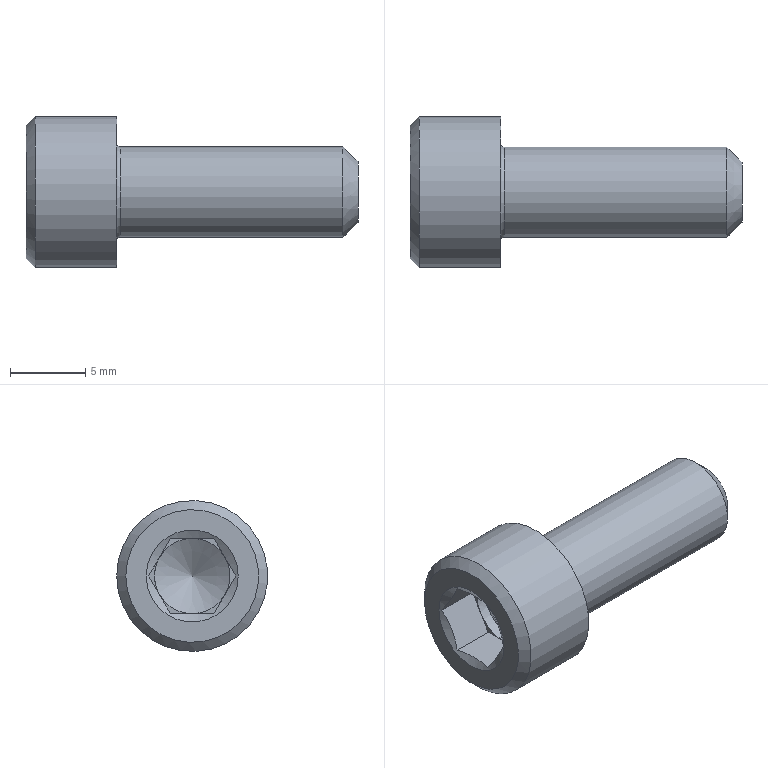Part | STEP file | Винт М6-6gx16 ГОСТ 11738-84 | 1 solid | 23 faces | box 22 x 10 x 10 mm | volume 820.968 mm3 | plane 15 | cone 4 | cylinder 3 | torus 1 | commonest cylinder face diameters 5 x1 6 x1 10 x1
STEP:
#1=CARTESIAN_POINT('',(-6.,4.4,0.));
#2=VERTEX_POINT('',#1);
#3=CARTESIAN_POINT('',(-6.,0.,0.));
#4=DIRECTION('',(1.,0.,0.));
#5=DIRECTION('',(0.,1.,0.));
#6=AXIS2_PLACEMENT_3D('',#3,#4,#5);
#7=CIRCLE('',#6,4.4);
#8=EDGE_CURVE('',#2,#2,#7,.T.);
#9=ORIENTED_EDGE('',*,*,#8,.F.);
#10=EDGE_LOOP('',(#9));
#11=FACE_BOUND('',#10,.T.);
#12=CARTESIAN_POINT('',(-6.,3.05,0.));
#13=VERTEX_POINT('',#12);
#14=CARTESIAN_POINT('',(-6.,0.,0.));
#15=DIRECTION('',(1.,0.,0.));
#16=DIRECTION('',(0.,1.,0.));
#17=AXIS2_PLACEMENT_3D('',#14,#15,#16);
#18=CIRCLE('',#17,3.05);
#19=EDGE_CURVE('',#13,#13,#18,.T.);
#20=ORIENTED_EDGE('',*,*,#19,.T.);
#21=EDGE_LOOP('',(#20));
#22=FACE_BOUND('',#21,.T.);
#23=CARTESIAN_POINT('',(-6.,0.,0.));
#24=DIRECTION('',(-1.,0.,0.));
#25=DIRECTION('',(0.,1.,0.));
#26=AXIS2_PLACEMENT_3D('',#23,#24,#25);
#27=PLANE('',#26);
#28=ADVANCED_FACE('',(#11,#22),#27,.T.);
#29=CARTESIAN_POINT('',(-5.906,1.443,-2.5));
#30=VERTEX_POINT('',#29);
#31=CARTESIAN_POINT('',(-5.906,-1.443,-2.5));
#32=VERTEX_POINT('',#31);
#33=CARTESIAN_POINT('',(-5.906,1.443,-2.5));
#34=CARTESIAN_POINT('',(-5.9,1.424,-2.5));
#35=CARTESIAN_POINT('',(-5.89,1.389,-2.5));
#36=CARTESIAN_POINT('',(-5.88,1.351,-2.5));
#37=CARTESIAN_POINT('',(-5.867,1.304,-2.5));
#38=CARTESIAN_POINT('',(-5.848,1.232,-2.5));
#39=CARTESIAN_POINT('',(-5.827,1.146,-2.5));
#40=CARTESIAN_POINT('',(-5.803,1.043,-2.5));
#41=CARTESIAN_POINT('',(-5.774,0.909,-2.5));
#42=CARTESIAN_POINT('',(-5.75,0.7773,-2.5));
#43=CARTESIAN_POINT('',(-5.728,0.6356,-2.5));
#44=CARTESIAN_POINT('',(-5.711,0.5115,-2.5));
#45=CARTESIAN_POINT('',(-5.699,0.3892,-2.5));
#46=CARTESIAN_POINT('',(-5.692,0.2947,-2.5));
#47=CARTESIAN_POINT('',(-5.688,0.2222,-2.5));
#48=CARTESIAN_POINT('',(-5.684,0.1323,-2.5));
#49=CARTESIAN_POINT('',(-5.683,0.05578,-2.5));
#50=CARTESIAN_POINT('',(-5.682,-0.001577,-2.5));
#51=CARTESIAN_POINT('',(-5.683,-0.03169,-2.5));
#52=CARTESIAN_POINT('',(-5.683,-0.0738,-2.5));
#53=CARTESIAN_POINT('',(-5.684,-0.1276,-2.5));
#54=CARTESIAN_POINT('',(-5.687,-0.2055,-2.5));
#55=CARTESIAN_POINT('',(-5.692,-0.2839,-2.5));
#56=CARTESIAN_POINT('',(-5.696,-0.3444,-2.5));
#57=CARTESIAN_POINT('',(-5.7,-0.3959,-2.5));
#58=CARTESIAN_POINT('',(-5.705,-0.4472,-2.5));
#59=CARTESIAN_POINT('',(-5.713,-0.5148,-2.5));
#60=CARTESIAN_POINT('',(-5.722,-0.5907,-2.5));
#61=CARTESIAN_POINT('',(-5.73,-0.6507,-2.5));
#62=CARTESIAN_POINT('',(-5.738,-0.7005,-2.5));
#63=CARTESIAN_POINT('',(-5.746,-0.7498,-2.5));
#64=CARTESIAN_POINT('',(-5.757,-0.8136,-2.5));
#65=CARTESIAN_POINT('',(-5.77,-0.8864,-2.5));
#66=CARTESIAN_POINT('',(-5.785,-0.9583,-2.5));
#67=CARTESIAN_POINT('',(-5.8,-1.03,-2.5));
#68=CARTESIAN_POINT('',(-5.812,-1.084,-2.5));
#69=CARTESIAN_POINT('',(-5.823,-1.131,-2.5));
#70=CARTESIAN_POINT('',(-5.834,-1.177,-2.5));
#71=CARTESIAN_POINT('',(-5.85,-1.239,-2.5));
#72=CARTESIAN_POINT('',(-5.868,-1.307,-2.5));
#73=CARTESIAN_POINT('',(-5.882,-1.361,-2.5));
#74=CARTESIAN_POINT('',(-5.895,-1.406,-2.5));
#75=CARTESIAN_POINT('',(-5.902,-1.429,-2.5));
#76=CARTESIAN_POINT('',(-5.906,-1.443,-2.5));
#77=B_SPLINE_CURVE_WITH_KNOTS('',3,(#33,#34,#35,#36,#37,#38,#39,#40,#41,#42,#43,#44,#45,#46,#47,#48,#49,#50,#51,#52,#53,#54,#55,#56,#57,#58,#59,#60,#61,#62,#63,#64,#65,#66,#67,#68,#69,#70,#71,#72,#73,#74,#75,#76),.UNSPECIFIED.,.F.,.F.,(4,1,1,1,1,1,1,1,1,1,1,1,1,1,1,1,1,1,1,1,1,1,1,1,1,1,1,1,1,1,1,1,1,1,1,1,1,1,1,1,1,4),(0.,0.02097,0.03685,0.04095,0.07015,0.1134,0.1316,0.1778,0.2541,0.2686,0.3246,0.3823,0.3943,0.4217,0.4566,0.4863,0.5,0.5153,0.5171,0.5431,0.5703,0.5969,0.6234,0.6325,0.6498,0.6761,0.7022,0.7281,0.7381,0.7538,0.7792,0.8044,0.8294,0.8543,0.8789,0.8866,0.9033,0.9276,0.9518,0.9759,0.9843,1.),.UNSPECIFIED.);
#78=EDGE_CURVE('',#30,#32,#77,.T.);
#79=ORIENTED_EDGE('',*,*,#78,.T.);
#80=CARTESIAN_POINT('',(-3.,-1.443,-2.5));
#81=VERTEX_POINT('',#80);
#82=CARTESIAN_POINT('',(-3.,-1.443,-2.5));
#83=DIRECTION('',(-1.,0.,0.));
#84=VECTOR('',#83,1.);
#85=LINE('',#82,#84);
#86=EDGE_CURVE('',#81,#32,#85,.T.);
#87=ORIENTED_EDGE('',*,*,#86,.F.);
#88=CARTESIAN_POINT('',(-3.,0.,-2.5));
#89=VERTEX_POINT('',#88);
#90=CARTESIAN_POINT('',(-3.,0.,-2.5));
#91=DIRECTION('',(0.,-1.,0.));
#92=VECTOR('',#91,1.);
#93=LINE('',#90,#92);
#94=EDGE_CURVE('',#89,#81,#93,.T.);
#95=ORIENTED_EDGE('',*,*,#94,.F.);
#96=CARTESIAN_POINT('',(-3.,1.443,-2.5));
#97=VERTEX_POINT('',#96);
#98=CARTESIAN_POINT('',(-3.,1.443,-2.5));
#99=DIRECTION('',(0.,-1.,0.));
#100=VECTOR('',#99,1.);
#101=LINE('',#98,#100);
#102=EDGE_CURVE('',#97,#89,#101,.T.);
#103=ORIENTED_EDGE('',*,*,#102,.F.);
#104=CARTESIAN_POINT('',(-3.,1.443,-2.5));
#105=DIRECTION('',(-1.,0.,0.));
#106=VECTOR('',#105,1.);
#107=LINE('',#104,#106);
#108=EDGE_CURVE('',#97,#30,#107,.T.);
#109=ORIENTED_EDGE('',*,*,#108,.T.);
#110=EDGE_LOOP('',(#79,#87,#95,#103,#109));
#111=FACE_BOUND('',#110,.T.);
#112=CARTESIAN_POINT('',(-3.,1.443,-2.5));
#113=DIRECTION('',(0.,0.,-1.));
#114=DIRECTION('',(0.,-1.,0.));
#115=AXIS2_PLACEMENT_3D('',#112,#113,#114);
#116=PLANE('',#115);
#117=ADVANCED_FACE('',(#111),#116,.F.);
#118=CARTESIAN_POINT('',(-5.906,-2.887,0.));
#119=VERTEX_POINT('',#118);
#120=CARTESIAN_POINT('',(-5.906,-1.443,-2.5));
#121=CARTESIAN_POINT('',(-5.9,-1.453,-2.483));
#122=CARTESIAN_POINT('',(-5.889,-1.472,-2.45));
#123=CARTESIAN_POINT('',(-5.871,-1.505,-2.392));
#124=CARTESIAN_POINT('',(-5.848,-1.549,-2.317));
#125=CARTESIAN_POINT('',(-5.816,-1.614,-2.204));
#126=CARTESIAN_POINT('',(-5.777,-1.702,-2.052));
#127=CARTESIAN_POINT('',(-5.74,-1.803,-1.877));
#128=CARTESIAN_POINT('',(-5.713,-1.902,-1.705));
#129=CARTESIAN_POINT('',(-5.697,-1.984,-1.564));
#130=CARTESIAN_POINT('',(-5.688,-2.048,-1.453));
#131=CARTESIAN_POINT('',(-5.684,-2.099,-1.365));
#132=CARTESIAN_POINT('',(-5.683,-2.137,-1.298));
#133=CARTESIAN_POINT('',(-5.682,-2.166,-1.249));
#134=CARTESIAN_POINT('',(-5.683,-2.194,-1.201));
#135=CARTESIAN_POINT('',(-5.684,-2.228,-1.141));
#136=CARTESIAN_POINT('',(-5.687,-2.268,-1.072));
#137=CARTESIAN_POINT('',(-5.692,-2.307,-1.004));
#138=CARTESIAN_POINT('',(-5.697,-2.346,-0.9371));
#139=CARTESIAN_POINT('',(-5.704,-2.384,-0.8704));
#140=CARTESIAN_POINT('',(-5.713,-2.422,-0.8041));
#141=CARTESIAN_POINT('',(-5.722,-2.46,-0.7384));
#142=CARTESIAN_POINT('',(-5.733,-2.498,-0.6734));
#143=CARTESIAN_POINT('',(-5.744,-2.535,-0.609));
#144=CARTESIAN_POINT('',(-5.757,-2.572,-0.5454));
#145=CARTESIAN_POINT('',(-5.77,-2.608,-0.4824));
#146=CARTESIAN_POINT('',(-5.785,-2.644,-0.4201));
#147=CARTESIAN_POINT('',(-5.8,-2.68,-0.3584));
#148=CARTESIAN_POINT('',(-5.816,-2.715,-0.2974));
#149=CARTESIAN_POINT('',(-5.832,-2.75,-0.237));
#150=CARTESIAN_POINT('',(-5.85,-2.784,-0.1771));
#151=CARTESIAN_POINT('',(-5.868,-2.819,-0.1177));
#152=CARTESIAN_POINT('',(-5.886,-2.853,-0.05869));
#153=CARTESIAN_POINT('',(-5.899,-2.875,-0.01952));
#154=CARTESIAN_POINT('',(-5.906,-2.887,0.));
#155=B_SPLINE_CURVE_WITH_KNOTS('',3,(#120,#121,#122,#123,#124,#125,#126,#127,#128,#129,#130,#131,#132,#133,#134,#135,#136,#137,#138,#139,#140,#141,#142,#143,#144,#145,#146,#147,#148,#149,#150,#151,#152,#153,#154),.UNSPECIFIED.,.F.,.F.,(4,1,1,1,1,1,1,1,1,1,1,1,1,1,1,1,1,1,1,1,1,1,1,1,1,1,1,1,1,1,1,1,4),(0.,0.02097,0.04095,0.07015,0.1134,0.1778,0.2541,0.3246,0.3823,0.4217,0.4566,0.4863,0.5,0.5153,0.5431,0.5703,0.5969,0.6234,0.6498,0.6761,0.7022,0.7281,0.7538,0.7792,0.8044,0.8294,0.8543,0.8789,0.9033,0.9276,0.9518,0.9759,1.),.UNSPECIFIED.);
#156=EDGE_CURVE('',#32,#119,#155,.T.);
#157=ORIENTED_EDGE('',*,*,#156,.T.);
#158=CARTESIAN_POINT('',(-3.,-2.887,0.));
#159=VERTEX_POINT('',#158);
#160=CARTESIAN_POINT('',(-3.,-2.887,0.));
#161=DIRECTION('',(-1.,0.,0.));
#162=VECTOR('',#161,1.);
#163=LINE('',#160,#162);
#164=EDGE_CURVE('',#159,#119,#163,.T.);
#165=ORIENTED_EDGE('',*,*,#164,.F.);
#166=CARTESIAN_POINT('',(-3.,-2.165,-1.25));
#167=VERTEX_POINT('',#166);
#168=CARTESIAN_POINT('',(-3.,-2.165,-1.25));
#169=DIRECTION('',(0.,-0.5,0.866));
#170=VECTOR('',#169,1.);
#171=LINE('',#168,#170);
#172=EDGE_CURVE('',#167,#159,#171,.T.);
#173=ORIENTED_EDGE('',*,*,#172,.F.);
#174=CARTESIAN_POINT('',(-3.,-1.443,-2.5));
#175=DIRECTION('',(0.,-0.5,0.866));
#176=VECTOR('',#175,1.);
#177=LINE('',#174,#176);
#178=EDGE_CURVE('',#81,#167,#177,.T.);
#179=ORIENTED_EDGE('',*,*,#178,.F.);
#180=ORIENTED_EDGE('',*,*,#86,.T.);
#181=EDGE_LOOP('',(#157,#165,#173,#179,#180));
#182=FACE_BOUND('',#181,.T.);
#183=CARTESIAN_POINT('',(-3.,-1.443,-2.5));
#184=DIRECTION('',(0.,-0.866,-0.5));
#185=DIRECTION('',(0.,-0.5,0.866));
#186=AXIS2_PLACEMENT_3D('',#183,#184,#185);
#187=PLANE('',#186);
#188=ADVANCED_FACE('',(#182),#187,.F.);
#189=CARTESIAN_POINT('',(-5.906,-1.443,2.5));
#190=VERTEX_POINT('',#189);
#191=CARTESIAN_POINT('',(-5.906,-2.887,0.));
#192=CARTESIAN_POINT('',(-5.9,-2.877,0.01704));
#193=CARTESIAN_POINT('',(-5.889,-2.858,0.05036));
#194=CARTESIAN_POINT('',(-5.871,-2.825,0.1076));
#195=CARTESIAN_POINT('',(-5.848,-2.781,0.1832));
#196=CARTESIAN_POINT('',(-5.816,-2.716,0.2956));
#197=CARTESIAN_POINT('',(-5.777,-2.628,0.4476));
#198=CARTESIAN_POINT('',(-5.74,-2.527,0.6235));
#199=CARTESIAN_POINT('',(-5.713,-2.428,0.7948));
#200=CARTESIAN_POINT('',(-5.697,-2.346,0.936));
#201=CARTESIAN_POINT('',(-5.688,-2.282,1.047));
#202=CARTESIAN_POINT('',(-5.684,-2.231,1.135));
#203=CARTESIAN_POINT('',(-5.683,-2.193,1.202));
#204=CARTESIAN_POINT('',(-5.682,-2.164,1.251));
#205=CARTESIAN_POINT('',(-5.683,-2.137,1.299));
#206=CARTESIAN_POINT('',(-5.684,-2.102,1.359));
#207=CARTESIAN_POINT('',(-5.687,-2.062,1.428));
#208=CARTESIAN_POINT('',(-5.692,-2.023,1.496));
#209=CARTESIAN_POINT('',(-5.697,-1.984,1.563));
#210=CARTESIAN_POINT('',(-5.704,-1.946,1.63));
#211=CARTESIAN_POINT('',(-5.713,-1.908,1.696));
#212=CARTESIAN_POINT('',(-5.722,-1.87,1.762));
#213=CARTESIAN_POINT('',(-5.733,-1.832,1.827));
#214=CARTESIAN_POINT('',(-5.744,-1.795,1.891));
#215=CARTESIAN_POINT('',(-5.757,-1.758,1.955));
#216=CARTESIAN_POINT('',(-5.77,-1.722,2.018));
#217=CARTESIAN_POINT('',(-5.785,-1.686,2.08));
#218=CARTESIAN_POINT('',(-5.8,-1.65,2.142));
#219=CARTESIAN_POINT('',(-5.816,-1.615,2.203));
#220=CARTESIAN_POINT('',(-5.832,-1.58,2.263));
#221=CARTESIAN_POINT('',(-5.85,-1.546,2.323));
#222=CARTESIAN_POINT('',(-5.868,-1.511,2.382));
#223=CARTESIAN_POINT('',(-5.886,-1.477,2.441));
#224=CARTESIAN_POINT('',(-5.899,-1.455,2.48));
#225=CARTESIAN_POINT('',(-5.906,-1.443,2.5));
#226=B_SPLINE_CURVE_WITH_KNOTS('',3,(#191,#192,#193,#194,#195,#196,#197,#198,#199,#200,#201,#202,#203,#204,#205,#206,#207,#208,#209,#210,#211,#212,#213,#214,#215,#216,#217,#218,#219,#220,#221,#222,#223,#224,#225),.UNSPECIFIED.,.F.,.F.,(4,1,1,1,1,1,1,1,1,1,1,1,1,1,1,1,1,1,1,1,1,1,1,1,1,1,1,1,1,1,1,1,4),(0.,0.02097,0.04095,0.07015,0.1134,0.1778,0.2541,0.3246,0.3823,0.4217,0.4566,0.4863,0.5,0.5153,0.5431,0.5703,0.5969,0.6234,0.6498,0.6761,0.7022,0.7281,0.7538,0.7792,0.8044,0.8294,0.8543,0.8789,0.9033,0.9276,0.9518,0.9759,1.),.UNSPECIFIED.);
#227=EDGE_CURVE('',#119,#190,#226,.T.);
#228=ORIENTED_EDGE('',*,*,#227,.T.);
#229=CARTESIAN_POINT('',(-3.,-1.443,2.5));
#230=VERTEX_POINT('',#229);
#231=CARTESIAN_POINT('',(-3.,-1.443,2.5));
#232=DIRECTION('',(-1.,0.,0.));
#233=VECTOR('',#232,1.);
#234=LINE('',#231,#233);
#235=EDGE_CURVE('',#230,#190,#234,.T.);
#236=ORIENTED_EDGE('',*,*,#235,.F.);
#237=CARTESIAN_POINT('',(-3.,-2.165,1.25));
#238=VERTEX_POINT('',#237);
#239=CARTESIAN_POINT('',(-3.,-2.165,1.25));
#240=DIRECTION('',(0.,0.5,0.866));
#241=VECTOR('',#240,1.);
#242=LINE('',#239,#241);
#243=EDGE_CURVE('',#238,#230,#242,.T.);
#244=ORIENTED_EDGE('',*,*,#243,.F.);
#245=CARTESIAN_POINT('',(-3.,-2.887,0.));
#246=DIRECTION('',(0.,0.5,0.866));
#247=VECTOR('',#246,1.);
#248=LINE('',#245,#247);
#249=EDGE_CURVE('',#159,#238,#248,.T.);
#250=ORIENTED_EDGE('',*,*,#249,.F.);
#251=ORIENTED_EDGE('',*,*,#164,.T.);
#252=EDGE_LOOP('',(#228,#236,#244,#250,#251));
#253=FACE_BOUND('',#252,.T.);
#254=CARTESIAN_POINT('',(-3.,-2.887,0.));
#255=DIRECTION('',(0.,-0.866,0.5));
#256=DIRECTION('',(0.,0.5,0.866));
#257=AXIS2_PLACEMENT_3D('',#254,#255,#256);
#258=PLANE('',#257);
#259=ADVANCED_FACE('',(#253),#258,.F.);
#260=CARTESIAN_POINT('',(-5.906,1.443,2.5));
#261=VERTEX_POINT('',#260);
#262=CARTESIAN_POINT('',(-5.906,-1.443,2.5));
#263=CARTESIAN_POINT('',(-5.9,-1.424,2.5));
#264=CARTESIAN_POINT('',(-5.89,-1.389,2.5));
#265=CARTESIAN_POINT('',(-5.88,-1.351,2.5));
#266=CARTESIAN_POINT('',(-5.867,-1.304,2.5));
#267=CARTESIAN_POINT('',(-5.848,-1.232,2.5));
#268=CARTESIAN_POINT('',(-5.827,-1.146,2.5));
#269=CARTESIAN_POINT('',(-5.803,-1.043,2.5));
#270=CARTESIAN_POINT('',(-5.774,-0.909,2.5));
#271=CARTESIAN_POINT('',(-5.75,-0.7773,2.5));
#272=CARTESIAN_POINT('',(-5.728,-0.6356,2.5));
#273=CARTESIAN_POINT('',(-5.711,-0.5115,2.5));
#274=CARTESIAN_POINT('',(-5.699,-0.3892,2.5));
#275=CARTESIAN_POINT('',(-5.692,-0.2947,2.5));
#276=CARTESIAN_POINT('',(-5.688,-0.2222,2.5));
#277=CARTESIAN_POINT('',(-5.684,-0.1323,2.5));
#278=CARTESIAN_POINT('',(-5.683,-0.05578,2.5));
#279=CARTESIAN_POINT('',(-5.682,0.001577,2.5));
#280=CARTESIAN_POINT('',(-5.683,0.03169,2.5));
#281=CARTESIAN_POINT('',(-5.683,0.0738,2.5));
#282=CARTESIAN_POINT('',(-5.684,0.1276,2.5));
#283=CARTESIAN_POINT('',(-5.687,0.2055,2.5));
#284=CARTESIAN_POINT('',(-5.692,0.2839,2.5));
#285=CARTESIAN_POINT('',(-5.696,0.3444,2.5));
#286=CARTESIAN_POINT('',(-5.7,0.3959,2.5));
#287=CARTESIAN_POINT('',(-5.705,0.4472,2.5));
#288=CARTESIAN_POINT('',(-5.713,0.5148,2.5));
#289=CARTESIAN_POINT('',(-5.722,0.5907,2.5));
#290=CARTESIAN_POINT('',(-5.73,0.6507,2.5));
#291=CARTESIAN_POINT('',(-5.738,0.7005,2.5));
#292=CARTESIAN_POINT('',(-5.746,0.7498,2.5));
#293=CARTESIAN_POINT('',(-5.757,0.8136,2.5));
#294=CARTESIAN_POINT('',(-5.77,0.8864,2.5));
#295=CARTESIAN_POINT('',(-5.785,0.9583,2.5));
#296=CARTESIAN_POINT('',(-5.8,1.03,2.5));
#297=CARTESIAN_POINT('',(-5.812,1.084,2.5));
#298=CARTESIAN_POINT('',(-5.823,1.131,2.5));
#299=CARTESIAN_POINT('',(-5.834,1.177,2.5));
#300=CARTESIAN_POINT('',(-5.85,1.239,2.5));
#301=CARTESIAN_POINT('',(-5.868,1.307,2.5));
#302=CARTESIAN_POINT('',(-5.882,1.361,2.5));
#303=CARTESIAN_POINT('',(-5.895,1.406,2.5));
#304=CARTESIAN_POINT('',(-5.902,1.429,2.5));
#305=CARTESIAN_POINT('',(-5.906,1.443,2.5));
#306=B_SPLINE_CURVE_WITH_KNOTS('',3,(#262,#263,#264,#265,#266,#267,#268,#269,#270,#271,#272,#273,#274,#275,#276,#277,#278,#279,#280,#281,#282,#283,#284,#285,#286,#287,#288,#289,#290,#291,#292,#293,#294,#295,#296,#297,#298,#299,#300,#301,#302,#303,#304,#305),.UNSPECIFIED.,.F.,.F.,(4,1,1,1,1,1,1,1,1,1,1,1,1,1,1,1,1,1,1,1,1,1,1,1,1,1,1,1,1,1,1,1,1,1,1,1,1,1,1,1,1,4),(0.,0.02097,0.03685,0.04095,0.07015,0.1134,0.1316,0.1778,0.2541,0.2686,0.3246,0.3823,0.3943,0.4217,0.4566,0.4863,0.5,0.5153,0.5171,0.5431,0.5703,0.5969,0.6234,0.6325,0.6498,0.6761,0.7022,0.7281,0.7381,0.7538,0.7792,0.8044,0.8294,0.8543,0.8789,0.8866,0.9033,0.9276,0.9518,0.9759,0.9843,1.),.UNSPECIFIED.);
#307=EDGE_CURVE('',#190,#261,#306,.T.);
#308=ORIENTED_EDGE('',*,*,#307,.T.);
#309=CARTESIAN_POINT('',(-3.,1.443,2.5));
#310=VERTEX_POINT('',#309);
#311=CARTESIAN_POINT('',(-3.,1.443,2.5));
#312=DIRECTION('',(-1.,0.,0.));
#313=VECTOR('',#312,1.);
#314=LINE('',#311,#313);
#315=EDGE_CURVE('',#310,#261,#314,.T.);
#316=ORIENTED_EDGE('',*,*,#315,.F.);
#317=CARTESIAN_POINT('',(-3.,0.,2.5));
#318=VERTEX_POINT('',#317);
#319=CARTESIAN_POINT('',(-3.,0.,2.5));
#320=DIRECTION('',(0.,1.,0.));
#321=VECTOR('',#320,1.);
#322=LINE('',#319,#321);
#323=EDGE_CURVE('',#318,#310,#322,.T.);
#324=ORIENTED_EDGE('',*,*,#323,.F.);
#325=CARTESIAN_POINT('',(-3.,-1.443,2.5));
#326=DIRECTION('',(0.,1.,0.));
#327=VECTOR('',#326,1.);
#328=LINE('',#325,#327);
#329=EDGE_CURVE('',#230,#318,#328,.T.);
#330=ORIENTED_EDGE('',*,*,#329,.F.);
#331=ORIENTED_EDGE('',*,*,#235,.T.);
#332=EDGE_LOOP('',(#308,#316,#324,#330,#331));
#333=FACE_BOUND('',#332,.T.);
#334=CARTESIAN_POINT('',(-3.,-1.443,2.5));
#335=DIRECTION('',(0.,0.,1.));
#336=DIRECTION('',(0.,1.,0.));
#337=AXIS2_PLACEMENT_3D('',#334,#335,#336);
#338=PLANE('',#337);
#339=ADVANCED_FACE('',(#333),#338,.F.);
#340=CARTESIAN_POINT('',(-5.906,2.887,0.));
#341=VERTEX_POINT('',#340);
#342=CARTESIAN_POINT('',(-5.906,2.887,0.));
#343=CARTESIAN_POINT('',(-5.9,2.877,-0.01704));
#344=CARTESIAN_POINT('',(-5.889,2.858,-0.05036));
#345=CARTESIAN_POINT('',(-5.871,2.825,-0.1076));
#346=CARTESIAN_POINT('',(-5.848,2.781,-0.1832));
#347=CARTESIAN_POINT('',(-5.816,2.716,-0.2956));
#348=CARTESIAN_POINT('',(-5.777,2.628,-0.4476));
#349=CARTESIAN_POINT('',(-5.74,2.527,-0.6235));
#350=CARTESIAN_POINT('',(-5.713,2.428,-0.7948));
#351=CARTESIAN_POINT('',(-5.697,2.346,-0.936));
#352=CARTESIAN_POINT('',(-5.688,2.282,-1.047));
#353=CARTESIAN_POINT('',(-5.684,2.231,-1.135));
#354=CARTESIAN_POINT('',(-5.683,2.193,-1.202));
#355=CARTESIAN_POINT('',(-5.682,2.164,-1.251));
#356=CARTESIAN_POINT('',(-5.683,2.137,-1.299));
#357=CARTESIAN_POINT('',(-5.684,2.102,-1.359));
#358=CARTESIAN_POINT('',(-5.687,2.062,-1.428));
#359=CARTESIAN_POINT('',(-5.692,2.023,-1.496));
#360=CARTESIAN_POINT('',(-5.697,1.984,-1.563));
#361=CARTESIAN_POINT('',(-5.704,1.946,-1.63));
#362=CARTESIAN_POINT('',(-5.713,1.908,-1.696));
#363=CARTESIAN_POINT('',(-5.722,1.87,-1.762));
#364=CARTESIAN_POINT('',(-5.733,1.832,-1.827));
#365=CARTESIAN_POINT('',(-5.744,1.795,-1.891));
#366=CARTESIAN_POINT('',(-5.757,1.758,-1.955));
#367=CARTESIAN_POINT('',(-5.77,1.722,-2.018));
#368=CARTESIAN_POINT('',(-5.785,1.686,-2.08));
#369=CARTESIAN_POINT('',(-5.8,1.65,-2.142));
#370=CARTESIAN_POINT('',(-5.816,1.615,-2.203));
#371=CARTESIAN_POINT('',(-5.832,1.58,-2.263));
#372=CARTESIAN_POINT('',(-5.85,1.546,-2.323));
#373=CARTESIAN_POINT('',(-5.868,1.511,-2.382));
#374=CARTESIAN_POINT('',(-5.886,1.477,-2.441));
#375=CARTESIAN_POINT('',(-5.899,1.455,-2.48));
#376=CARTESIAN_POINT('',(-5.906,1.443,-2.5));
#377=B_SPLINE_CURVE_WITH_KNOTS('',3,(#342,#343,#344,#345,#346,#347,#348,#349,#350,#351,#352,#353,#354,#355,#356,#357,#358,#359,#360,#361,#362,#363,#364,#365,#366,#367,#368,#369,#370,#371,#372,#373,#374,#375,#376),.UNSPECIFIED.,.F.,.F.,(4,1,1,1,1,1,1,1,1,1,1,1,1,1,1,1,1,1,1,1,1,1,1,1,1,1,1,1,1,1,1,1,4),(0.,0.02097,0.04095,0.07015,0.1134,0.1778,0.2541,0.3246,0.3823,0.4217,0.4566,0.4863,0.5,0.5153,0.5431,0.5703,0.5969,0.6234,0.6498,0.6761,0.7022,0.7281,0.7538,0.7792,0.8044,0.8294,0.8543,0.8789,0.9033,0.9276,0.9518,0.9759,1.),.UNSPECIFIED.);
#378=EDGE_CURVE('',#341,#30,#377,.T.);
#379=ORIENTED_EDGE('',*,*,#378,.T.);
#380=ORIENTED_EDGE('',*,*,#108,.F.);
#381=CARTESIAN_POINT('',(-3.,2.165,-1.25));
#382=VERTEX_POINT('',#381);
#383=CARTESIAN_POINT('',(-3.,2.165,-1.25));
#384=DIRECTION('',(0.,-0.5,-0.866));
#385=VECTOR('',#384,1.);
#386=LINE('',#383,#385);
#387=EDGE_CURVE('',#382,#97,#386,.T.);
#388=ORIENTED_EDGE('',*,*,#387,.F.);
#389=CARTESIAN_POINT('',(-3.,2.887,0.));
#390=VERTEX_POINT('',#389);
#391=CARTESIAN_POINT('',(-3.,2.887,0.));
#392=DIRECTION('',(0.,-0.5,-0.866));
#393=VECTOR('',#392,1.);
#394=LINE('',#391,#393);
#395=EDGE_CURVE('',#390,#382,#394,.T.);
#396=ORIENTED_EDGE('',*,*,#395,.F.);
#397=CARTESIAN_POINT('',(-3.,2.887,0.));
#398=DIRECTION('',(-1.,0.,0.));
#399=VECTOR('',#398,1.);
#400=LINE('',#397,#399);
#401=EDGE_CURVE('',#390,#341,#400,.T.);
#402=ORIENTED_EDGE('',*,*,#401,.T.);
#403=EDGE_LOOP('',(#379,#380,#388,#396,#402));
#404=FACE_BOUND('',#403,.T.);
#405=CARTESIAN_POINT('',(-3.,2.887,0.));
#406=DIRECTION('',(0.,0.866,-0.5));
#407=DIRECTION('',(0.,-0.5,-0.866));
#408=AXIS2_PLACEMENT_3D('',#405,#406,#407);
#409=PLANE('',#408);
#410=ADVANCED_FACE('',(#404),#409,.F.);
#411=CARTESIAN_POINT('',(-5.906,1.443,2.5));
#412=CARTESIAN_POINT('',(-5.9,1.453,2.483));
#413=CARTESIAN_POINT('',(-5.889,1.472,2.45));
#414=CARTESIAN_POINT('',(-5.871,1.505,2.392));
#415=CARTESIAN_POINT('',(-5.848,1.549,2.317));
#416=CARTESIAN_POINT('',(-5.816,1.614,2.204));
#417=CARTESIAN_POINT('',(-5.777,1.702,2.052));
#418=CARTESIAN_POINT('',(-5.74,1.803,1.877));
#419=CARTESIAN_POINT('',(-5.713,1.902,1.705));
#420=CARTESIAN_POINT('',(-5.697,1.984,1.564));
#421=CARTESIAN_POINT('',(-5.688,2.048,1.453));
#422=CARTESIAN_POINT('',(-5.684,2.099,1.365));
#423=CARTESIAN_POINT('',(-5.683,2.137,1.298));
#424=CARTESIAN_POINT('',(-5.682,2.166,1.249));
#425=CARTESIAN_POINT('',(-5.683,2.194,1.201));
#426=CARTESIAN_POINT('',(-5.684,2.228,1.141));
#427=CARTESIAN_POINT('',(-5.687,2.268,1.072));
#428=CARTESIAN_POINT('',(-5.692,2.307,1.004));
#429=CARTESIAN_POINT('',(-5.697,2.346,0.9371));
#430=CARTESIAN_POINT('',(-5.704,2.384,0.8704));
#431=CARTESIAN_POINT('',(-5.713,2.422,0.8041));
#432=CARTESIAN_POINT('',(-5.722,2.46,0.7384));
#433=CARTESIAN_POINT('',(-5.733,2.498,0.6734));
#434=CARTESIAN_POINT('',(-5.744,2.535,0.609));
#435=CARTESIAN_POINT('',(-5.757,2.572,0.5454));
#436=CARTESIAN_POINT('',(-5.77,2.608,0.4824));
#437=CARTESIAN_POINT('',(-5.785,2.644,0.4201));
#438=CARTESIAN_POINT('',(-5.8,2.68,0.3584));
#439=CARTESIAN_POINT('',(-5.816,2.715,0.2974));
#440=CARTESIAN_POINT('',(-5.832,2.75,0.237));
#441=CARTESIAN_POINT('',(-5.85,2.784,0.1771));
#442=CARTESIAN_POINT('',(-5.868,2.819,0.1177));
#443=CARTESIAN_POINT('',(-5.886,2.853,0.05869));
#444=CARTESIAN_POINT('',(-5.899,2.875,0.01952));
#445=CARTESIAN_POINT('',(-5.906,2.887,0.));
#446=B_SPLINE_CURVE_WITH_KNOTS('',3,(#411,#412,#413,#414,#415,#416,#417,#418,#419,#420,#421,#422,#423,#424,#425,#426,#427,#428,#429,#430,#431,#432,#433,#434,#435,#436,#437,#438,#439,#440,#441,#442,#443,#444,#445),.UNSPECIFIED.,.F.,.F.,(4,1,1,1,1,1,1,1,1,1,1,1,1,1,1,1,1,1,1,1,1,1,1,1,1,1,1,1,1,1,1,1,4),(0.,0.02097,0.04095,0.07015,0.1134,0.1778,0.2541,0.3246,0.3823,0.4217,0.4566,0.4863,0.5,0.5153,0.5431,0.5703,0.5969,0.6234,0.6498,0.6761,0.7022,0.7281,0.7538,0.7792,0.8044,0.8294,0.8543,0.8789,0.9033,0.9276,0.9518,0.9759,1.),.UNSPECIFIED.);
#447=EDGE_CURVE('',#261,#341,#446,.T.);
#448=ORIENTED_EDGE('',*,*,#447,.T.);
#449=ORIENTED_EDGE('',*,*,#401,.F.);
#450=CARTESIAN_POINT('',(-3.,2.165,1.25));
#451=VERTEX_POINT('',#450);
#452=CARTESIAN_POINT('',(-3.,2.165,1.25));
#453=DIRECTION('',(0.,0.5,-0.866));
#454=VECTOR('',#453,1.);
#455=LINE('',#452,#454);
#456=EDGE_CURVE('',#451,#390,#455,.T.);
#457=ORIENTED_EDGE('',*,*,#456,.F.);
#458=CARTESIAN_POINT('',(-3.,1.443,2.5));
#459=DIRECTION('',(0.,0.5,-0.866));
#460=VECTOR('',#459,1.);
#461=LINE('',#458,#460);
#462=EDGE_CURVE('',#310,#451,#461,.T.);
#463=ORIENTED_EDGE('',*,*,#462,.F.);
#464=ORIENTED_EDGE('',*,*,#315,.T.);
#465=EDGE_LOOP('',(#448,#449,#457,#463,#464));
#466=FACE_BOUND('',#465,.T.);
#467=CARTESIAN_POINT('',(-3.,1.443,2.5));
#468=DIRECTION('',(0.,0.866,0.5));
#469=DIRECTION('',(0.,0.5,-0.866));
#470=AXIS2_PLACEMENT_3D('',#467,#468,#469);
#471=PLANE('',#470);
#472=ADVANCED_FACE('',(#466),#471,.F.);
#473=ORIENTED_EDGE('',*,*,#447,.F.);
#474=ORIENTED_EDGE('',*,*,#307,.F.);
#475=ORIENTED_EDGE('',*,*,#227,.F.);
#476=ORIENTED_EDGE('',*,*,#156,.F.);
#477=ORIENTED_EDGE('',*,*,#78,.F.);
#478=ORIENTED_EDGE('',*,*,#378,.F.);
#479=EDGE_LOOP('',(#473,#474,#475,#476,#477,#478));
#480=FACE_BOUND('',#479,.T.);
#481=ORIENTED_EDGE('',*,*,#19,.F.);
#482=EDGE_LOOP('',(#481));
#483=FACE_OUTER_BOUND('',#482,.T.);
#484=CARTESIAN_POINT('',(-5.841,0.,0.));
#485=DIRECTION('',(-1.,0.,0.));
#486=DIRECTION('',(0.,-1.,0.));
#487=AXIS2_PLACEMENT_3D('',#484,#485,#486);
#488=CONICAL_SURFACE('',#487,2.775,1.047);
#489=ADVANCED_FACE('',(#480,#483),#488,.F.);
#490=CARTESIAN_POINT('',(-5.4,5.,0.));
#491=VERTEX_POINT('',#490);
#492=CARTESIAN_POINT('',(-5.4,0.,0.));
#493=DIRECTION('',(1.,0.,0.));
#494=DIRECTION('',(0.,1.,0.));
#495=AXIS2_PLACEMENT_3D('',#492,#493,#494);
#496=CIRCLE('',#495,5.);
#497=EDGE_CURVE('',#491,#491,#496,.T.);
#498=ORIENTED_EDGE('',*,*,#497,.F.);
#499=EDGE_LOOP('',(#498));
#500=FACE_OUTER_BOUND('',#499,.T.);
#501=ORIENTED_EDGE('',*,*,#8,.T.);
#502=EDGE_LOOP('',(#501));
#503=FACE_OUTER_BOUND('',#502,.T.);
#504=CARTESIAN_POINT('',(-5.7,0.,0.));
#505=DIRECTION('',(1.,0.,0.));
#506=DIRECTION('',(0.,1.,0.));
#507=AXIS2_PLACEMENT_3D('',#504,#505,#506);
#508=CONICAL_SURFACE('',#507,4.7,0.7854);
#509=ADVANCED_FACE('',(#500,#503),#508,.T.);
#510=CARTESIAN_POINT('',(-3.,0.,0.));
#511=DIRECTION('',(1.,0.,0.));
#512=DIRECTION('',(0.,-0.866,-0.5));
#513=AXIS2_PLACEMENT_3D('',#510,#511,#512);
#514=CIRCLE('',#513,2.5);
#515=EDGE_CURVE('',#167,#89,#514,.T.);
#516=ORIENTED_EDGE('',*,*,#515,.T.);
#517=ORIENTED_EDGE('',*,*,#94,.T.);
#518=ORIENTED_EDGE('',*,*,#178,.T.);
#519=EDGE_LOOP('',(#516,#517,#518));
#520=FACE_BOUND('',#519,.T.);
#521=CARTESIAN_POINT('',(-3.,0.,0.));
#522=DIRECTION('',(-1.,0.,0.));
#523=DIRECTION('',(0.,0.,-1.));
#524=AXIS2_PLACEMENT_3D('',#521,#522,#523);
#525=PLANE('',#524);
#526=ADVANCED_FACE('',(#520),#525,.T.);
#527=CARTESIAN_POINT('',(-3.,0.,0.));
#528=DIRECTION('',(1.,0.,0.));
#529=DIRECTION('',(0.,0.,-1.));
#530=AXIS2_PLACEMENT_3D('',#527,#528,#529);
#531=CIRCLE('',#530,2.5);
#532=EDGE_CURVE('',#89,#382,#531,.T.);
#533=ORIENTED_EDGE('',*,*,#532,.T.);
#534=ORIENTED_EDGE('',*,*,#387,.T.);
#535=ORIENTED_EDGE('',*,*,#102,.T.);
#536=EDGE_LOOP('',(#533,#534,#535));
#537=FACE_BOUND('',#536,.T.);
#538=CARTESIAN_POINT('',(-3.,0.,0.));
#539=DIRECTION('',(-1.,0.,0.));
#540=DIRECTION('',(0.,0.,-1.));
#541=AXIS2_PLACEMENT_3D('',#538,#539,#540);
#542=PLANE('',#541);
#543=ADVANCED_FACE('',(#537),#542,.T.);
#544=CARTESIAN_POINT('',(-3.,0.,0.));
#545=DIRECTION('',(1.,0.,0.));
#546=DIRECTION('',(0.,-0.866,0.5));
#547=AXIS2_PLACEMENT_3D('',#544,#545,#546);
#548=CIRCLE('',#547,2.5);
#549=EDGE_CURVE('',#238,#167,#548,.T.);
#550=ORIENTED_EDGE('',*,*,#549,.T.);
#551=ORIENTED_EDGE('',*,*,#172,.T.);
#552=ORIENTED_EDGE('',*,*,#249,.T.);
#553=EDGE_LOOP('',(#550,#551,#552));
#554=FACE_BOUND('',#553,.T.);
#555=CARTESIAN_POINT('',(-3.,0.,0.));
#556=DIRECTION('',(-1.,0.,0.));
#557=DIRECTION('',(0.,0.,-1.));
#558=AXIS2_PLACEMENT_3D('',#555,#556,#557);
#559=PLANE('',#558);
#560=ADVANCED_FACE('',(#554),#559,.T.);
#561=CARTESIAN_POINT('',(-3.,0.,0.));
#562=DIRECTION('',(1.,0.,0.));
#563=DIRECTION('',(0.,0.,1.));
#564=AXIS2_PLACEMENT_3D('',#561,#562,#563);
#565=CIRCLE('',#564,2.5);
#566=EDGE_CURVE('',#318,#238,#565,.T.);
#567=ORIENTED_EDGE('',*,*,#566,.T.);
#568=ORIENTED_EDGE('',*,*,#243,.T.);
#569=ORIENTED_EDGE('',*,*,#329,.T.);
#570=EDGE_LOOP('',(#567,#568,#569));
#571=FACE_BOUND('',#570,.T.);
#572=CARTESIAN_POINT('',(-3.,0.,0.));
#573=DIRECTION('',(-1.,0.,0.));
#574=DIRECTION('',(0.,0.,-1.));
#575=AXIS2_PLACEMENT_3D('',#572,#573,#574);
#576=PLANE('',#575);
#577=ADVANCED_FACE('',(#571),#576,.T.);
#578=CARTESIAN_POINT('',(-3.,0.,0.));
#579=DIRECTION('',(1.,0.,0.));
#580=DIRECTION('',(0.,0.866,0.5));
#581=AXIS2_PLACEMENT_3D('',#578,#579,#580);
#582=CIRCLE('',#581,2.5);
#583=EDGE_CURVE('',#451,#318,#582,.T.);
#584=ORIENTED_EDGE('',*,*,#583,.T.);
#585=ORIENTED_EDGE('',*,*,#323,.T.);
#586=ORIENTED_EDGE('',*,*,#462,.T.);
#587=EDGE_LOOP('',(#584,#585,#586));
#588=FACE_BOUND('',#587,.T.);
#589=CARTESIAN_POINT('',(-3.,0.,0.));
#590=DIRECTION('',(-1.,0.,0.));
#591=DIRECTION('',(0.,0.,-1.));
#592=AXIS2_PLACEMENT_3D('',#589,#590,#591);
#593=PLANE('',#592);
#594=ADVANCED_FACE('',(#588),#593,.T.);
#595=CARTESIAN_POINT('',(-3.,2.5,0.));
#596=VERTEX_POINT('',#595);
#597=CARTESIAN_POINT('',(-3.,0.,0.));
#598=DIRECTION('',(1.,0.,0.));
#599=DIRECTION('',(0.,1.,0.));
#600=AXIS2_PLACEMENT_3D('',#597,#598,#599);
#601=CIRCLE('',#600,2.5);
#602=EDGE_CURVE('',#596,#451,#601,.T.);
#603=ORIENTED_EDGE('',*,*,#602,.T.);
#604=ORIENTED_EDGE('',*,*,#456,.T.);
#605=ORIENTED_EDGE('',*,*,#395,.T.);
#606=CARTESIAN_POINT('',(-3.,0.,0.));
#607=DIRECTION('',(1.,0.,0.));
#608=DIRECTION('',(0.,0.866,-0.5));
#609=AXIS2_PLACEMENT_3D('',#606,#607,#608);
#610=CIRCLE('',#609,2.5);
#611=EDGE_CURVE('',#382,#596,#610,.T.);
#612=ORIENTED_EDGE('',*,*,#611,.T.);
#613=EDGE_LOOP('',(#603,#604,#605,#612));
#614=FACE_BOUND('',#613,.T.);
#615=CARTESIAN_POINT('',(-3.,0.,0.));
#616=DIRECTION('',(-1.,0.,0.));
#617=DIRECTION('',(0.,0.,-1.));
#618=AXIS2_PLACEMENT_3D('',#615,#616,#617);
#619=PLANE('',#618);
#620=ADVANCED_FACE('',(#614),#619,.T.);
#621=CARTESIAN_POINT('',(0.,5.,0.));
#622=VERTEX_POINT('',#621);
#623=CARTESIAN_POINT('',(0.,0.,0.));
#624=DIRECTION('',(1.,0.,0.));
#625=DIRECTION('',(0.,1.,0.));
#626=AXIS2_PLACEMENT_3D('',#623,#624,#625);
#627=CIRCLE('',#626,5.);
#628=EDGE_CURVE('',#622,#622,#627,.T.);
#629=ORIENTED_EDGE('',*,*,#628,.F.);
#630=EDGE_LOOP('',(#629));
#631=FACE_OUTER_BOUND('',#630,.T.);
#632=ORIENTED_EDGE('',*,*,#497,.T.);
#633=EDGE_LOOP('',(#632));
#634=FACE_OUTER_BOUND('',#633,.T.);
#635=CARTESIAN_POINT('',(-6.,0.,0.));
#636=DIRECTION('',(1.,0.,0.));
#637=DIRECTION('',(0.,1.,0.));
#638=AXIS2_PLACEMENT_3D('',#635,#636,#637);
#639=CYLINDRICAL_SURFACE('',#638,5.);
#640=ADVANCED_FACE('',(#631,#634),#639,.T.);
#641=CARTESIAN_POINT('',(-2.3,2.5,0.));
#642=VERTEX_POINT('',#641);
#643=CARTESIAN_POINT('',(-2.3,0.,0.));
#644=DIRECTION('',(1.,0.,0.));
#645=DIRECTION('',(0.,1.,0.));
#646=AXIS2_PLACEMENT_3D('',#643,#644,#645);
#647=CIRCLE('',#646,2.5);
#648=EDGE_CURVE('',#642,#642,#647,.T.);
#649=ORIENTED_EDGE('',*,*,#648,.T.);
#650=EDGE_LOOP('',(#649));
#651=FACE_OUTER_BOUND('',#650,.T.);
#652=ORIENTED_EDGE('',*,*,#611,.F.);
#653=ORIENTED_EDGE('',*,*,#532,.F.);
#654=ORIENTED_EDGE('',*,*,#515,.F.);
#655=ORIENTED_EDGE('',*,*,#549,.F.);
#656=ORIENTED_EDGE('',*,*,#566,.F.);
#657=ORIENTED_EDGE('',*,*,#583,.F.);
#658=ORIENTED_EDGE('',*,*,#602,.F.);
#659=EDGE_LOOP('',(#652,#653,#654,#655,#656,#657,#658));
#660=FACE_BOUND('',#659,.T.);
#661=CARTESIAN_POINT('',(-6.,0.,0.));
#662=DIRECTION('',(1.,0.,0.));
#663=DIRECTION('',(0.,1.,0.));
#664=AXIS2_PLACEMENT_3D('',#661,#662,#663);
#665=CYLINDRICAL_SURFACE('',#664,2.5);
#666=ADVANCED_FACE('',(#651,#660),#665,.F.);
#667=ORIENTED_EDGE('',*,*,#628,.T.);
#668=EDGE_LOOP('',(#667));
#669=FACE_BOUND('',#668,.T.);
#670=CARTESIAN_POINT('',(0.,0.,-3.25));
#671=VERTEX_POINT('',#670);
#672=CARTESIAN_POINT('',(0.,0.,0.));
#673=DIRECTION('',(-1.,0.,0.));
#674=DIRECTION('',(0.,0.,-1.));
#675=AXIS2_PLACEMENT_3D('',#672,#673,#674);
#676=CIRCLE('',#675,3.25);
#677=EDGE_CURVE('',#671,#671,#676,.T.);
#678=ORIENTED_EDGE('',*,*,#677,.T.);
#679=EDGE_LOOP('',(#678));
#680=FACE_BOUND('',#679,.T.);
#681=CARTESIAN_POINT('',(0.,0.,0.));
#682=DIRECTION('',(1.,0.,0.));
#683=DIRECTION('',(0.,1.,0.));
#684=AXIS2_PLACEMENT_3D('',#681,#682,#683);
#685=PLANE('',#684);
#686=ADVANCED_FACE('',(#669,#680),#685,.T.);
#687=ORIENTED_EDGE('',*,*,#648,.F.);
#688=EDGE_LOOP('',(#687));
#689=FACE_OUTER_BOUND('',#688,.T.);
#690=CARTESIAN_POINT('',(-1.578,0.,0.));
#691=DIRECTION('',(-1.,0.,0.));
#692=DIRECTION('',(0.,-1.,0.));
#693=AXIS2_PLACEMENT_3D('',#690,#691,#692);
#694=CONICAL_SURFACE('',#693,1.25,1.047);
#695=ADVANCED_FACE('',(#689),#694,.F.);
#696=CARTESIAN_POINT('',(0.25,0.,-3.));
#697=VERTEX_POINT('',#696);
#698=CARTESIAN_POINT('',(0.25,0.,0.));
#699=DIRECTION('',(-1.,0.,0.));
#700=DIRECTION('',(0.,0.,-1.));
#701=AXIS2_PLACEMENT_3D('',#698,#699,#700);
#702=CIRCLE('',#701,3.);
#703=EDGE_CURVE('',#697,#697,#702,.T.);
#704=ORIENTED_EDGE('',*,*,#703,.T.);
#705=EDGE_LOOP('',(#704));
#706=FACE_OUTER_BOUND('',#705,.T.);
#707=ORIENTED_EDGE('',*,*,#677,.F.);
#708=EDGE_LOOP('',(#707));
#709=FACE_OUTER_BOUND('',#708,.T.);
#710=CARTESIAN_POINT('',(0.25,0.,0.));
#711=DIRECTION('',(-1.,0.,0.));
#712=DIRECTION('',(0.,0.,-1.));
#713=AXIS2_PLACEMENT_3D('',#710,#711,#712);
#714=TOROIDAL_SURFACE('',#713,3.25,0.25);
#715=ADVANCED_FACE('',(#706,#709),#714,.F.);
#716=CARTESIAN_POINT('',(15.,0.,-3.));
#717=VERTEX_POINT('',#716);
#718=CARTESIAN_POINT('',(15.,0.,0.));
#719=DIRECTION('',(-1.,0.,0.));
#720=DIRECTION('',(0.,0.,-1.));
#721=AXIS2_PLACEMENT_3D('',#718,#719,#720);
#722=CIRCLE('',#721,3.);
#723=EDGE_CURVE('',#717,#717,#722,.T.);
#724=ORIENTED_EDGE('',*,*,#723,.T.);
#725=EDGE_LOOP('',(#724));
#726=FACE_OUTER_BOUND('',#725,.T.);
#727=ORIENTED_EDGE('',*,*,#703,.F.);
#728=EDGE_LOOP('',(#727));
#729=FACE_OUTER_BOUND('',#728,.T.);
#730=CARTESIAN_POINT('',(16.,0.,0.));
#731=DIRECTION('',(-1.,0.,0.));
#732=DIRECTION('',(0.,0.,-1.));
#733=AXIS2_PLACEMENT_3D('',#730,#731,#732);
#734=CYLINDRICAL_SURFACE('',#733,3.);
#735=ADVANCED_FACE('',(#726,#729),#734,.T.);
#736=CARTESIAN_POINT('',(16.,0.,-2.));
#737=VERTEX_POINT('',#736);
#738=CARTESIAN_POINT('',(16.,0.,0.));
#739=DIRECTION('',(-1.,0.,0.));
#740=DIRECTION('',(0.,0.,-1.));
#741=AXIS2_PLACEMENT_3D('',#738,#739,#740);
#742=CIRCLE('',#741,2.);
#743=EDGE_CURVE('',#737,#737,#742,.T.);
#744=ORIENTED_EDGE('',*,*,#743,.F.);
#745=EDGE_LOOP('',(#744));
#746=FACE_BOUND('',#745,.T.);
#747=CARTESIAN_POINT('',(16.,0.,0.));
#748=DIRECTION('',(-1.,0.,0.));
#749=DIRECTION('',(0.,0.,-1.));
#750=AXIS2_PLACEMENT_3D('',#747,#748,#749);
#751=PLANE('',#750);
#752=ADVANCED_FACE('',(#746),#751,.F.);
#753=ORIENTED_EDGE('',*,*,#743,.T.);
#754=EDGE_LOOP('',(#753));
#755=FACE_OUTER_BOUND('',#754,.T.);
#756=ORIENTED_EDGE('',*,*,#723,.F.);
#757=EDGE_LOOP('',(#756));
#758=FACE_OUTER_BOUND('',#757,.T.);
#759=CARTESIAN_POINT('',(15.5,0.,0.));
#760=DIRECTION('',(-1.,0.,0.));
#761=DIRECTION('',(0.,0.,-1.));
#762=AXIS2_PLACEMENT_3D('',#759,#760,#761);
#763=CONICAL_SURFACE('',#762,2.5,0.7854);
#764=ADVANCED_FACE('',(#755,#758),#763,.T.);
#765=CLOSED_SHELL('',(#28,#117,#188,#259,#339,#410,#472,#489,#509,#526,#543,#560,#577,#594,#620,#640,#666,#686,#695,#715,#735,#752,#764));
#766=MANIFOLD_SOLID_BREP('',#765);
#767=(LENGTH_UNIT()NAMED_UNIT(*)SI_UNIT(.MILLI.,.METRE.));
#768=UNCERTAINTY_MEASURE_WITH_UNIT(LENGTH_MEASURE(0.00001),#767,'','');
#769=(NAMED_UNIT(*)PLANE_ANGLE_UNIT()SI_UNIT($,.RADIAN.));
#770=(NAMED_UNIT(*)SI_UNIT($,.STERADIAN.)SOLID_ANGLE_UNIT());
#771=(GEOMETRIC_REPRESENTATION_CONTEXT(3)GLOBAL_UNCERTAINTY_ASSIGNED_CONTEXT((#768))GLOBAL_UNIT_ASSIGNED_CONTEXT((#767,#769,#770))REPRESENTATION_CONTEXT('',''));
#772=ADVANCED_BREP_SHAPE_REPRESENTATION('',(#766),#771);